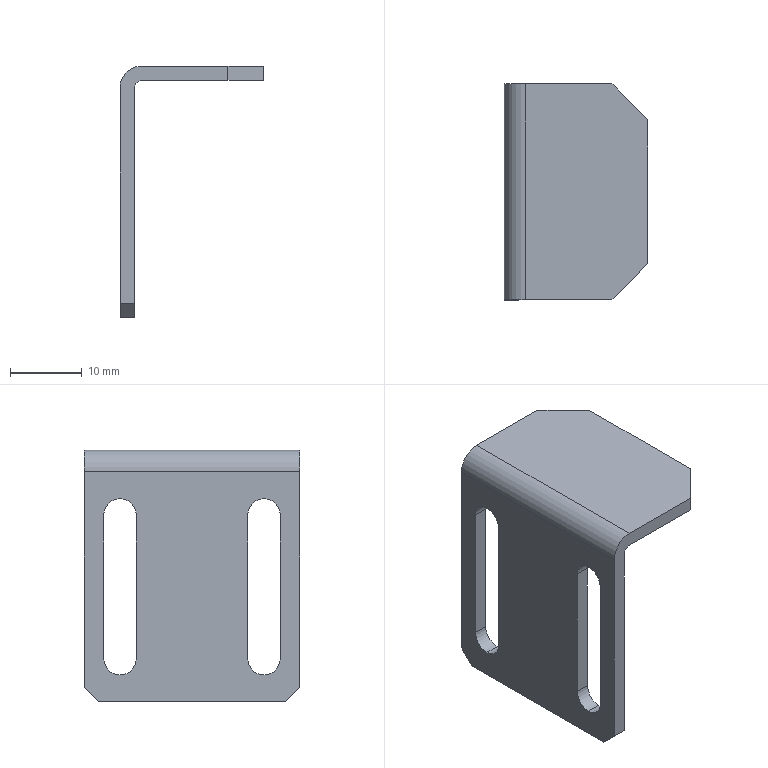Part | SolidWorks | features Chamfer 2, Fillet 2, ICE 2, Extrusion 1 | 1 solid | 24 faces | box 20 x 30 x 35 mm | volume 2647 mm3 | plane 16 | cylinder 8 | commonest cylinder face diameters 4.5 x6 2 x1 6 x1
STEP:
#1=CARTESIAN_POINT('',(0.,5.,-31.25));
#2=VERTEX_POINT('',#1);
#3=CARTESIAN_POINT('',(0.,7.25,-29.));
#4=VERTEX_POINT('',#3);
#5=CARTESIAN_POINT('',(0.,5.,-29.));
#6=DIRECTION('',(1.,0.,0.));
#7=DIRECTION('',(0.,0.,-1.));
#8=AXIS2_PLACEMENT_3D('',#5,#6,#7);
#9=CIRCLE('',#8,2.25);
#10=EDGE_CURVE('',#2,#4,#9,.T.);
#11=ORIENTED_EDGE('',*,*,#10,.F.);
#12=CARTESIAN_POINT('',(2.,5.,-31.25));
#13=VERTEX_POINT('',#12);
#14=CARTESIAN_POINT('',(-8.,5.,-31.25));
#15=DIRECTION('',(1.,0.,0.));
#16=VECTOR('',#15,1000.);
#17=LINE('',#14,#16);
#18=EDGE_CURVE('',#2,#13,#17,.T.);
#19=ORIENTED_EDGE('',*,*,#18,.T.);
#20=CARTESIAN_POINT('',(2.,7.25,-29.));
#21=VERTEX_POINT('',#20);
#22=CARTESIAN_POINT('',(2.,5.,-29.));
#23=DIRECTION('',(1.,0.,0.));
#24=DIRECTION('',(0.,0.,1.));
#25=AXIS2_PLACEMENT_3D('',#22,#23,#24);
#26=CIRCLE('',#25,2.25);
#27=EDGE_CURVE('',#13,#21,#26,.T.);
#28=ORIENTED_EDGE('',*,*,#27,.T.);
#29=CARTESIAN_POINT('',(-8.,7.25,-29.));
#30=DIRECTION('',(-1.,0.,0.));
#31=VECTOR('',#30,1000.);
#32=LINE('',#29,#31);
#33=EDGE_CURVE('',#21,#4,#32,.T.);
#34=ORIENTED_EDGE('',*,*,#33,.T.);
#35=EDGE_LOOP('',(#11,#19,#28,#34));
#36=FACE_OUTER_BOUND('',#35,.T.);
#37=CARTESIAN_POINT('',(-8.,5.,-29.));
#38=DIRECTION('',(1.,0.,0.));
#39=DIRECTION('',(0.,0.,-1.));
#40=AXIS2_PLACEMENT_3D('',#37,#38,#39);
#41=CYLINDRICAL_SURFACE('',#40,2.25);
#42=ADVANCED_FACE('',(#36),#41,.F.);
#43=CARTESIAN_POINT('',(0.,25.,-31.25));
#44=VERTEX_POINT('',#43);
#45=CARTESIAN_POINT('',(0.,27.25,-29.));
#46=VERTEX_POINT('',#45);
#47=CARTESIAN_POINT('',(0.,25.,-29.));
#48=DIRECTION('',(1.,0.,0.));
#49=DIRECTION('',(0.,0.,-1.));
#50=AXIS2_PLACEMENT_3D('',#47,#48,#49);
#51=CIRCLE('',#50,2.25);
#52=EDGE_CURVE('',#44,#46,#51,.T.);
#53=ORIENTED_EDGE('',*,*,#52,.F.);
#54=CARTESIAN_POINT('',(2.,25.,-31.25));
#55=VERTEX_POINT('',#54);
#56=CARTESIAN_POINT('',(-8.,25.,-31.25));
#57=DIRECTION('',(1.,0.,0.));
#58=VECTOR('',#57,1000.);
#59=LINE('',#56,#58);
#60=EDGE_CURVE('',#44,#55,#59,.T.);
#61=ORIENTED_EDGE('',*,*,#60,.T.);
#62=CARTESIAN_POINT('',(2.,27.25,-29.));
#63=VERTEX_POINT('',#62);
#64=CARTESIAN_POINT('',(2.,25.,-29.));
#65=DIRECTION('',(1.,0.,0.));
#66=DIRECTION('',(0.,0.,-1.));
#67=AXIS2_PLACEMENT_3D('',#64,#65,#66);
#68=CIRCLE('',#67,2.25);
#69=EDGE_CURVE('',#55,#63,#68,.T.);
#70=ORIENTED_EDGE('',*,*,#69,.T.);
#71=CARTESIAN_POINT('',(-8.,27.25,-29.));
#72=DIRECTION('',(-1.,0.,0.));
#73=VECTOR('',#72,1000.);
#74=LINE('',#71,#73);
#75=EDGE_CURVE('',#63,#46,#74,.T.);
#76=ORIENTED_EDGE('',*,*,#75,.T.);
#77=EDGE_LOOP('',(#53,#61,#70,#76));
#78=FACE_OUTER_BOUND('',#77,.T.);
#79=CARTESIAN_POINT('',(-8.,25.,-29.));
#80=DIRECTION('',(1.,0.,0.));
#81=DIRECTION('',(0.,0.,-1.));
#82=AXIS2_PLACEMENT_3D('',#79,#80,#81);
#83=CYLINDRICAL_SURFACE('',#82,2.25);
#84=ADVANCED_FACE('',(#78),#83,.F.);
#85=ORIENTED_EDGE('',*,*,#60,.F.);
#86=CARTESIAN_POINT('',(0.,22.75,-29.));
#87=VERTEX_POINT('',#86);
#88=CARTESIAN_POINT('',(0.,25.,-29.));
#89=DIRECTION('',(1.,0.,0.));
#90=DIRECTION('',(0.,0.,-1.));
#91=AXIS2_PLACEMENT_3D('',#88,#89,#90);
#92=CIRCLE('',#91,2.25);
#93=EDGE_CURVE('',#87,#44,#92,.T.);
#94=ORIENTED_EDGE('',*,*,#93,.F.);
#95=CARTESIAN_POINT('',(2.,22.75,-29.));
#96=VERTEX_POINT('',#95);
#97=CARTESIAN_POINT('',(-8.,22.75,-29.));
#98=DIRECTION('',(-1.,0.,0.));
#99=VECTOR('',#98,1000.);
#100=LINE('',#97,#99);
#101=EDGE_CURVE('',#96,#87,#100,.T.);
#102=ORIENTED_EDGE('',*,*,#101,.F.);
#103=CARTESIAN_POINT('',(2.,25.,-29.));
#104=DIRECTION('',(1.,0.,0.));
#105=DIRECTION('',(0.,0.,-1.));
#106=AXIS2_PLACEMENT_3D('',#103,#104,#105);
#107=CIRCLE('',#106,2.25);
#108=EDGE_CURVE('',#96,#55,#107,.T.);
#109=ORIENTED_EDGE('',*,*,#108,.T.);
#110=EDGE_LOOP('',(#85,#94,#102,#109));
#111=FACE_OUTER_BOUND('',#110,.T.);
#112=CARTESIAN_POINT('',(-8.,25.,-29.));
#113=DIRECTION('',(1.,0.,0.));
#114=DIRECTION('',(0.,0.,-1.));
#115=AXIS2_PLACEMENT_3D('',#112,#113,#114);
#116=CYLINDRICAL_SURFACE('',#115,2.25);
#117=ADVANCED_FACE('',(#111),#116,.F.);
#118=ORIENTED_EDGE('',*,*,#18,.F.);
#119=CARTESIAN_POINT('',(0.,2.75,-29.));
#120=VERTEX_POINT('',#119);
#121=CARTESIAN_POINT('',(0.,5.,-29.));
#122=DIRECTION('',(1.,0.,0.));
#123=DIRECTION('',(0.,0.,-1.));
#124=AXIS2_PLACEMENT_3D('',#121,#122,#123);
#125=CIRCLE('',#124,2.25);
#126=EDGE_CURVE('',#120,#2,#125,.T.);
#127=ORIENTED_EDGE('',*,*,#126,.F.);
#128=CARTESIAN_POINT('',(2.,2.75,-29.));
#129=VERTEX_POINT('',#128);
#130=CARTESIAN_POINT('',(-8.,2.75,-29.));
#131=DIRECTION('',(-1.,0.,0.));
#132=VECTOR('',#131,1000.);
#133=LINE('',#130,#132);
#134=EDGE_CURVE('',#129,#120,#133,.T.);
#135=ORIENTED_EDGE('',*,*,#134,.F.);
#136=CARTESIAN_POINT('',(2.,5.,-29.));
#137=DIRECTION('',(1.,0.,0.));
#138=DIRECTION('',(0.,0.,1.));
#139=AXIS2_PLACEMENT_3D('',#136,#137,#138);
#140=CIRCLE('',#139,2.25);
#141=EDGE_CURVE('',#129,#13,#140,.T.);
#142=ORIENTED_EDGE('',*,*,#141,.T.);
#143=EDGE_LOOP('',(#118,#127,#135,#142));
#144=FACE_OUTER_BOUND('',#143,.T.);
#145=CARTESIAN_POINT('',(-8.,5.,-29.));
#146=DIRECTION('',(1.,0.,0.));
#147=DIRECTION('',(0.,0.,-1.));
#148=AXIS2_PLACEMENT_3D('',#145,#146,#147);
#149=CYLINDRICAL_SURFACE('',#148,2.25);
#150=ADVANCED_FACE('',(#144),#149,.F.);
#151=CARTESIAN_POINT('',(0.,7.25,-9.));
#152=VERTEX_POINT('',#151);
#153=CARTESIAN_POINT('',(0.,2.75,-9.));
#154=VERTEX_POINT('',#153);
#155=CARTESIAN_POINT('',(0.,5.,-9.));
#156=DIRECTION('',(1.,0.,0.));
#157=DIRECTION('',(0.,0.,-1.));
#158=AXIS2_PLACEMENT_3D('',#155,#156,#157);
#159=CIRCLE('',#158,2.25);
#160=EDGE_CURVE('',#152,#154,#159,.T.);
#161=ORIENTED_EDGE('',*,*,#160,.T.);
#162=CARTESIAN_POINT('',(0.,2.75,0.));
#163=DIRECTION('',(0.,0.,-1.));
#164=VECTOR('',#163,1000.);
#165=LINE('',#162,#164);
#166=EDGE_CURVE('',#154,#120,#165,.T.);
#167=ORIENTED_EDGE('',*,*,#166,.T.);
#168=ORIENTED_EDGE('',*,*,#126,.T.);
#169=ORIENTED_EDGE('',*,*,#10,.T.);
#170=CARTESIAN_POINT('',(0.,7.25,0.));
#171=DIRECTION('',(0.,0.,1.));
#172=VECTOR('',#171,1000.);
#173=LINE('',#170,#172);
#174=EDGE_CURVE('',#4,#152,#173,.T.);
#175=ORIENTED_EDGE('',*,*,#174,.T.);
#176=EDGE_LOOP('',(#161,#167,#168,#169,#175));
#177=FACE_BOUND('',#176,.T.);
#178=CARTESIAN_POINT('',(0.,27.25,-9.));
#179=VERTEX_POINT('',#178);
#180=CARTESIAN_POINT('',(0.,22.75,-9.));
#181=VERTEX_POINT('',#180);
#182=CARTESIAN_POINT('',(0.,25.,-9.));
#183=DIRECTION('',(1.,0.,0.));
#184=DIRECTION('',(0.,0.,-1.));
#185=AXIS2_PLACEMENT_3D('',#182,#183,#184);
#186=CIRCLE('',#185,2.25);
#187=EDGE_CURVE('',#179,#181,#186,.T.);
#188=ORIENTED_EDGE('',*,*,#187,.T.);
#189=CARTESIAN_POINT('',(0.,22.75,0.));
#190=DIRECTION('',(0.,0.,-1.));
#191=VECTOR('',#190,1000.);
#192=LINE('',#189,#191);
#193=EDGE_CURVE('',#181,#87,#192,.T.);
#194=ORIENTED_EDGE('',*,*,#193,.T.);
#195=ORIENTED_EDGE('',*,*,#93,.T.);
#196=ORIENTED_EDGE('',*,*,#52,.T.);
#197=CARTESIAN_POINT('',(0.,27.25,0.));
#198=DIRECTION('',(0.,0.,1.));
#199=VECTOR('',#198,1000.);
#200=LINE('',#197,#199);
#201=EDGE_CURVE('',#46,#179,#200,.T.);
#202=ORIENTED_EDGE('',*,*,#201,.T.);
#203=EDGE_LOOP('',(#188,#194,#195,#196,#202));
#204=FACE_BOUND('',#203,.T.);
#205=CARTESIAN_POINT('',(0.,0.,-33.));
#206=VERTEX_POINT('',#205);
#207=CARTESIAN_POINT('',(0.,0.,-3.));
#208=VERTEX_POINT('',#207);
#209=CARTESIAN_POINT('',(0.,0.,0.));
#210=DIRECTION('',(0.,0.,1.));
#211=VECTOR('',#210,1000.);
#212=LINE('',#209,#211);
#213=EDGE_CURVE('',#206,#208,#212,.T.);
#214=ORIENTED_EDGE('',*,*,#213,.T.);
#215=CARTESIAN_POINT('',(0.,30.,-3.));
#216=VERTEX_POINT('',#215);
#217=CARTESIAN_POINT('',(0.,30.,-3.));
#218=DIRECTION('',(0.,1.,0.));
#219=VECTOR('',#218,1000.);
#220=LINE('',#217,#219);
#221=EDGE_CURVE('',#208,#216,#220,.T.);
#222=ORIENTED_EDGE('',*,*,#221,.T.);
#223=CARTESIAN_POINT('',(0.,30.,-33.));
#224=VERTEX_POINT('',#223);
#225=CARTESIAN_POINT('',(0.,30.,0.));
#226=DIRECTION('',(0.,0.,1.));
#227=VECTOR('',#226,1000.);
#228=LINE('',#225,#227);
#229=EDGE_CURVE('',#224,#216,#228,.T.);
#230=ORIENTED_EDGE('',*,*,#229,.F.);
#231=CARTESIAN_POINT('',(0.,28.,-35.));
#232=VERTEX_POINT('',#231);
#233=CARTESIAN_POINT('',(0.,30.,-33.));
#234=DIRECTION('',(0.,-0.7071,-0.7071));
#235=VECTOR('',#234,1000.);
#236=LINE('',#233,#235);
#237=EDGE_CURVE('',#224,#232,#236,.T.);
#238=ORIENTED_EDGE('',*,*,#237,.T.);
#239=CARTESIAN_POINT('',(0.,2.,-35.));
#240=VERTEX_POINT('',#239);
#241=CARTESIAN_POINT('',(0.,30.,-35.));
#242=DIRECTION('',(0.,-1.,0.));
#243=VECTOR('',#242,1000.);
#244=LINE('',#241,#243);
#245=EDGE_CURVE('',#232,#240,#244,.T.);
#246=ORIENTED_EDGE('',*,*,#245,.T.);
#247=CARTESIAN_POINT('',(0.,2.,-35.));
#248=DIRECTION('',(0.,-0.7071,0.7071));
#249=VECTOR('',#248,1000.);
#250=LINE('',#247,#249);
#251=EDGE_CURVE('',#240,#206,#250,.T.);
#252=ORIENTED_EDGE('',*,*,#251,.T.);
#253=EDGE_LOOP('',(#214,#222,#230,#238,#246,#252));
#254=FACE_OUTER_BOUND('',#253,.T.);
#255=CARTESIAN_POINT('',(0.,30.,0.));
#256=DIRECTION('',(1.,0.,0.));
#257=DIRECTION('',(0.,0.,-1.));
#258=AXIS2_PLACEMENT_3D('',#255,#256,#257);
#259=PLANE('',#258);
#260=ADVANCED_FACE('',(#177,#204,#254),#259,.F.);
#261=CARTESIAN_POINT('',(20.,25.,0.));
#262=VERTEX_POINT('',#261);
#263=CARTESIAN_POINT('',(20.,5.,0.));
#264=VERTEX_POINT('',#263);
#265=CARTESIAN_POINT('',(20.,30.,0.));
#266=DIRECTION('',(0.,-1.,0.));
#267=VECTOR('',#266,1000.);
#268=LINE('',#265,#267);
#269=EDGE_CURVE('',#262,#264,#268,.T.);
#270=ORIENTED_EDGE('',*,*,#269,.F.);
#271=CARTESIAN_POINT('',(15.,30.,0.));
#272=VERTEX_POINT('',#271);
#273=CARTESIAN_POINT('',(15.,30.,0.));
#274=DIRECTION('',(-0.7071,0.7071,0.));
#275=VECTOR('',#274,1000.);
#276=LINE('',#273,#275);
#277=EDGE_CURVE('',#262,#272,#276,.T.);
#278=ORIENTED_EDGE('',*,*,#277,.T.);
#279=CARTESIAN_POINT('',(3.,30.,0.));
#280=VERTEX_POINT('',#279);
#281=CARTESIAN_POINT('',(0.,30.,0.));
#282=DIRECTION('',(1.,0.,0.));
#283=VECTOR('',#282,1000.);
#284=LINE('',#281,#283);
#285=EDGE_CURVE('',#280,#272,#284,.T.);
#286=ORIENTED_EDGE('',*,*,#285,.F.);
#287=CARTESIAN_POINT('',(3.,0.,0.));
#288=VERTEX_POINT('',#287);
#289=CARTESIAN_POINT('',(3.,30.,0.));
#290=DIRECTION('',(0.,-1.,0.));
#291=VECTOR('',#290,1000.);
#292=LINE('',#289,#291);
#293=EDGE_CURVE('',#280,#288,#292,.T.);
#294=ORIENTED_EDGE('',*,*,#293,.T.);
#295=CARTESIAN_POINT('',(15.,0.,0.));
#296=VERTEX_POINT('',#295);
#297=CARTESIAN_POINT('',(0.,0.,0.));
#298=DIRECTION('',(1.,0.,0.));
#299=VECTOR('',#298,1000.);
#300=LINE('',#297,#299);
#301=EDGE_CURVE('',#288,#296,#300,.T.);
#302=ORIENTED_EDGE('',*,*,#301,.T.);
#303=CARTESIAN_POINT('',(20.,5.,0.));
#304=DIRECTION('',(0.7071,0.7071,0.));
#305=VECTOR('',#304,1000.);
#306=LINE('',#303,#305);
#307=EDGE_CURVE('',#296,#264,#306,.T.);
#308=ORIENTED_EDGE('',*,*,#307,.T.);
#309=EDGE_LOOP('',(#270,#278,#286,#294,#302,#308));
#310=FACE_OUTER_BOUND('',#309,.T.);
#311=CARTESIAN_POINT('',(0.,30.,0.));
#312=DIRECTION('',(0.,0.,-1.));
#313=DIRECTION('',(-1.,0.,0.));
#314=AXIS2_PLACEMENT_3D('',#311,#312,#313);
#315=PLANE('',#314);
#316=ADVANCED_FACE('',(#310),#315,.F.);
#317=CARTESIAN_POINT('',(20.,25.,-2.));
#318=VERTEX_POINT('',#317);
#319=CARTESIAN_POINT('',(20.,5.,-2.));
#320=VERTEX_POINT('',#319);
#321=CARTESIAN_POINT('',(20.,30.,-2.));
#322=DIRECTION('',(0.,-1.,0.));
#323=VECTOR('',#322,1000.);
#324=LINE('',#321,#323);
#325=EDGE_CURVE('',#318,#320,#324,.T.);
#326=ORIENTED_EDGE('',*,*,#325,.F.);
#327=CARTESIAN_POINT('',(20.,25.,0.));
#328=DIRECTION('',(0.,0.,1.));
#329=VECTOR('',#328,1000.);
#330=LINE('',#327,#329);
#331=EDGE_CURVE('',#318,#262,#330,.T.);
#332=ORIENTED_EDGE('',*,*,#331,.T.);
#333=ORIENTED_EDGE('',*,*,#269,.T.);
#334=CARTESIAN_POINT('',(20.,5.,-2.));
#335=DIRECTION('',(0.,0.,-1.));
#336=VECTOR('',#335,1000.);
#337=LINE('',#334,#336);
#338=EDGE_CURVE('',#264,#320,#337,.T.);
#339=ORIENTED_EDGE('',*,*,#338,.T.);
#340=EDGE_LOOP('',(#326,#332,#333,#339));
#341=FACE_OUTER_BOUND('',#340,.T.);
#342=CARTESIAN_POINT('',(20.,30.,0.));
#343=DIRECTION('',(-1.,0.,0.));
#344=DIRECTION('',(0.,0.,1.));
#345=AXIS2_PLACEMENT_3D('',#342,#343,#344);
#346=PLANE('',#345);
#347=ADVANCED_FACE('',(#341),#346,.F.);
#348=CARTESIAN_POINT('',(15.,30.,-2.));
#349=VERTEX_POINT('',#348);
#350=CARTESIAN_POINT('',(3.,30.,-2.));
#351=VERTEX_POINT('',#350);
#352=CARTESIAN_POINT('',(20.,30.,-2.));
#353=DIRECTION('',(-1.,0.,0.));
#354=VECTOR('',#353,1000.);
#355=LINE('',#352,#354);
#356=EDGE_CURVE('',#349,#351,#355,.T.);
#357=ORIENTED_EDGE('',*,*,#356,.F.);
#358=CARTESIAN_POINT('',(15.,30.,-2.));
#359=DIRECTION('',(0.7071,-0.7071,0.));
#360=VECTOR('',#359,1000.);
#361=LINE('',#358,#360);
#362=EDGE_CURVE('',#349,#318,#361,.T.);
#363=ORIENTED_EDGE('',*,*,#362,.T.);
#364=ORIENTED_EDGE('',*,*,#325,.T.);
#365=CARTESIAN_POINT('',(15.,0.,-2.));
#366=VERTEX_POINT('',#365);
#367=CARTESIAN_POINT('',(20.,5.,-2.));
#368=DIRECTION('',(-0.7071,-0.7071,0.));
#369=VECTOR('',#368,1000.);
#370=LINE('',#367,#369);
#371=EDGE_CURVE('',#320,#366,#370,.T.);
#372=ORIENTED_EDGE('',*,*,#371,.T.);
#373=CARTESIAN_POINT('',(3.,0.,-2.));
#374=VERTEX_POINT('',#373);
#375=CARTESIAN_POINT('',(20.,0.,-2.));
#376=DIRECTION('',(-1.,0.,0.));
#377=VECTOR('',#376,1000.);
#378=LINE('',#375,#377);
#379=EDGE_CURVE('',#366,#374,#378,.T.);
#380=ORIENTED_EDGE('',*,*,#379,.T.);
#381=CARTESIAN_POINT('',(3.,30.,-2.));
#382=DIRECTION('',(0.,1.,0.));
#383=VECTOR('',#382,1000.);
#384=LINE('',#381,#383);
#385=EDGE_CURVE('',#374,#351,#384,.T.);
#386=ORIENTED_EDGE('',*,*,#385,.T.);
#387=EDGE_LOOP('',(#357,#363,#364,#372,#380,#386));
#388=FACE_OUTER_BOUND('',#387,.T.);
#389=CARTESIAN_POINT('',(20.,30.,-2.));
#390=DIRECTION('',(0.,0.,1.));
#391=DIRECTION('',(1.,0.,0.));
#392=AXIS2_PLACEMENT_3D('',#389,#390,#391);
#393=PLANE('',#392);
#394=ADVANCED_FACE('',(#388),#393,.F.);
#395=ORIENTED_EDGE('',*,*,#141,.F.);
#396=CARTESIAN_POINT('',(2.,2.75,-9.));
#397=VERTEX_POINT('',#396);
#398=CARTESIAN_POINT('',(2.,2.75,-29.));
#399=DIRECTION('',(0.,0.,-1.));
#400=VECTOR('',#399,1000.);
#401=LINE('',#398,#400);
#402=EDGE_CURVE('',#397,#129,#401,.T.);
#403=ORIENTED_EDGE('',*,*,#402,.F.);
#404=CARTESIAN_POINT('',(2.,7.25,-9.));
#405=VERTEX_POINT('',#404);
#406=CARTESIAN_POINT('',(2.,5.,-9.));
#407=DIRECTION('',(1.,0.,0.));
#408=DIRECTION('',(0.,0.,-1.));
#409=AXIS2_PLACEMENT_3D('',#406,#407,#408);
#410=CIRCLE('',#409,2.25);
#411=EDGE_CURVE('',#405,#397,#410,.T.);
#412=ORIENTED_EDGE('',*,*,#411,.F.);
#413=CARTESIAN_POINT('',(2.,7.25,-29.));
#414=DIRECTION('',(0.,0.,1.));
#415=VECTOR('',#414,1000.);
#416=LINE('',#413,#415);
#417=EDGE_CURVE('',#21,#405,#416,.T.);
#418=ORIENTED_EDGE('',*,*,#417,.F.);
#419=ORIENTED_EDGE('',*,*,#27,.F.);
#420=EDGE_LOOP('',(#395,#403,#412,#418,#419));
#421=FACE_BOUND('',#420,.T.);
#422=ORIENTED_EDGE('',*,*,#108,.F.);
#423=CARTESIAN_POINT('',(2.,22.75,-9.));
#424=VERTEX_POINT('',#423);
#425=CARTESIAN_POINT('',(2.,22.75,-29.));
#426=DIRECTION('',(0.,0.,-1.));
#427=VECTOR('',#426,1000.);
#428=LINE('',#425,#427);
#429=EDGE_CURVE('',#424,#96,#428,.T.);
#430=ORIENTED_EDGE('',*,*,#429,.F.);
#431=CARTESIAN_POINT('',(2.,27.25,-9.));
#432=VERTEX_POINT('',#431);
#433=CARTESIAN_POINT('',(2.,25.,-9.));
#434=DIRECTION('',(1.,0.,0.));
#435=DIRECTION('',(0.,0.,1.));
#436=AXIS2_PLACEMENT_3D('',#433,#434,#435);
#437=CIRCLE('',#436,2.25);
#438=EDGE_CURVE('',#432,#424,#437,.T.);
#439=ORIENTED_EDGE('',*,*,#438,.F.);
#440=CARTESIAN_POINT('',(2.,27.25,-29.));
#441=DIRECTION('',(0.,0.,1.));
#442=VECTOR('',#441,1000.);
#443=LINE('',#440,#442);
#444=EDGE_CURVE('',#63,#432,#443,.T.);
#445=ORIENTED_EDGE('',*,*,#444,.F.);
#446=ORIENTED_EDGE('',*,*,#69,.F.);
#447=EDGE_LOOP('',(#422,#430,#439,#445,#446));
#448=FACE_BOUND('',#447,.T.);
#449=CARTESIAN_POINT('',(2.,30.,-3.));
#450=VERTEX_POINT('',#449);
#451=CARTESIAN_POINT('',(2.,30.,-33.));
#452=VERTEX_POINT('',#451);
#453=CARTESIAN_POINT('',(2.,30.,-35.));
#454=DIRECTION('',(0.,0.,-1.));
#455=VECTOR('',#454,1000.);
#456=LINE('',#453,#455);
#457=EDGE_CURVE('',#450,#452,#456,.T.);
#458=ORIENTED_EDGE('',*,*,#457,.F.);
#459=CARTESIAN_POINT('',(2.,0.,-3.));
#460=VERTEX_POINT('',#459);
#461=CARTESIAN_POINT('',(2.,0.,-3.));
#462=DIRECTION('',(0.,-1.,0.));
#463=VECTOR('',#462,1000.);
#464=LINE('',#461,#463);
#465=EDGE_CURVE('',#450,#460,#464,.T.);
#466=ORIENTED_EDGE('',*,*,#465,.T.);
#467=CARTESIAN_POINT('',(2.,0.,-33.));
#468=VERTEX_POINT('',#467);
#469=CARTESIAN_POINT('',(2.,0.,-35.));
#470=DIRECTION('',(0.,0.,-1.));
#471=VECTOR('',#470,1000.);
#472=LINE('',#469,#471);
#473=EDGE_CURVE('',#460,#468,#472,.T.);
#474=ORIENTED_EDGE('',*,*,#473,.T.);
#475=CARTESIAN_POINT('',(2.,2.,-35.));
#476=VERTEX_POINT('',#475);
#477=CARTESIAN_POINT('',(2.,2.,-35.));
#478=DIRECTION('',(0.,0.7071,-0.7071));
#479=VECTOR('',#478,1000.);
#480=LINE('',#477,#479);
#481=EDGE_CURVE('',#468,#476,#480,.T.);
#482=ORIENTED_EDGE('',*,*,#481,.T.);
#483=CARTESIAN_POINT('',(2.,28.,-35.));
#484=VERTEX_POINT('',#483);
#485=CARTESIAN_POINT('',(2.,30.,-35.));
#486=DIRECTION('',(0.,-1.,0.));
#487=VECTOR('',#486,1000.);
#488=LINE('',#485,#487);
#489=EDGE_CURVE('',#484,#476,#488,.T.);
#490=ORIENTED_EDGE('',*,*,#489,.F.);
#491=CARTESIAN_POINT('',(2.,30.,-33.));
#492=DIRECTION('',(0.,0.7071,0.7071));
#493=VECTOR('',#492,1000.);
#494=LINE('',#491,#493);
#495=EDGE_CURVE('',#484,#452,#494,.T.);
#496=ORIENTED_EDGE('',*,*,#495,.T.);
#497=EDGE_LOOP('',(#458,#466,#474,#482,#490,#496));
#498=FACE_OUTER_BOUND('',#497,.T.);
#499=CARTESIAN_POINT('',(2.,30.,-35.));
#500=DIRECTION('',(-1.,0.,0.));
#501=DIRECTION('',(0.,0.,1.));
#502=AXIS2_PLACEMENT_3D('',#499,#500,#501);
#503=PLANE('',#502);
#504=ADVANCED_FACE('',(#421,#448,#498),#503,.F.);
#505=ORIENTED_EDGE('',*,*,#245,.F.);
#506=CARTESIAN_POINT('',(0.,28.,-35.));
#507=DIRECTION('',(1.,0.,0.));
#508=VECTOR('',#507,1000.);
#509=LINE('',#506,#508);
#510=EDGE_CURVE('',#232,#484,#509,.T.);
#511=ORIENTED_EDGE('',*,*,#510,.T.);
#512=ORIENTED_EDGE('',*,*,#489,.T.);
#513=CARTESIAN_POINT('',(0.,2.,-35.));
#514=DIRECTION('',(-1.,0.,0.));
#515=VECTOR('',#514,1000.);
#516=LINE('',#513,#515);
#517=EDGE_CURVE('',#476,#240,#516,.T.);
#518=ORIENTED_EDGE('',*,*,#517,.T.);
#519=EDGE_LOOP('',(#505,#511,#512,#518));
#520=FACE_OUTER_BOUND('',#519,.T.);
#521=CARTESIAN_POINT('',(0.,30.,-35.));
#522=DIRECTION('',(0.,0.,1.));
#523=DIRECTION('',(1.,0.,0.));
#524=AXIS2_PLACEMENT_3D('',#521,#522,#523);
#525=PLANE('',#524);
#526=ADVANCED_FACE('',(#520),#525,.F.);
#527=ORIENTED_EDGE('',*,*,#285,.T.);
#528=CARTESIAN_POINT('',(15.,30.,0.));
#529=DIRECTION('',(0.,0.,-1.));
#530=VECTOR('',#529,1000.);
#531=LINE('',#528,#530);
#532=EDGE_CURVE('',#272,#349,#531,.T.);
#533=ORIENTED_EDGE('',*,*,#532,.T.);
#534=ORIENTED_EDGE('',*,*,#356,.T.);
#535=CARTESIAN_POINT('',(3.,30.,-3.));
#536=DIRECTION('',(0.,-1.,0.));
#537=DIRECTION('',(0.,0.,-1.));
#538=AXIS2_PLACEMENT_3D('',#535,#536,#537);
#539=CIRCLE('',#538,1.);
#540=EDGE_CURVE('',#351,#450,#539,.T.);
#541=ORIENTED_EDGE('',*,*,#540,.T.);
#542=ORIENTED_EDGE('',*,*,#457,.T.);
#543=CARTESIAN_POINT('',(0.,30.,-33.));
#544=DIRECTION('',(-1.,0.,0.));
#545=VECTOR('',#544,1000.);
#546=LINE('',#543,#545);
#547=EDGE_CURVE('',#452,#224,#546,.T.);
#548=ORIENTED_EDGE('',*,*,#547,.T.);
#549=ORIENTED_EDGE('',*,*,#229,.T.);
#550=CARTESIAN_POINT('',(3.,30.,-3.));
#551=DIRECTION('',(0.,1.,0.));
#552=DIRECTION('',(0.,0.,-1.));
#553=AXIS2_PLACEMENT_3D('',#550,#551,#552);
#554=CIRCLE('',#553,3.);
#555=EDGE_CURVE('',#216,#280,#554,.T.);
#556=ORIENTED_EDGE('',*,*,#555,.T.);
#557=EDGE_LOOP('',(#527,#533,#534,#541,#542,#548,#549,#556));
#558=FACE_OUTER_BOUND('',#557,.T.);
#559=CARTESIAN_POINT('',(0.,30.,0.));
#560=DIRECTION('',(0.,-1.,0.));
#561=DIRECTION('',(0.,0.,-1.));
#562=AXIS2_PLACEMENT_3D('',#559,#560,#561);
#563=PLANE('',#562);
#564=ADVANCED_FACE('',(#558),#563,.F.);
#565=ORIENTED_EDGE('',*,*,#379,.F.);
#566=CARTESIAN_POINT('',(15.,0.,0.));
#567=DIRECTION('',(0.,0.,1.));
#568=VECTOR('',#567,1000.);
#569=LINE('',#566,#568);
#570=EDGE_CURVE('',#366,#296,#569,.T.);
#571=ORIENTED_EDGE('',*,*,#570,.T.);
#572=ORIENTED_EDGE('',*,*,#301,.F.);
#573=CARTESIAN_POINT('',(3.,0.,-3.));
#574=DIRECTION('',(0.,-1.,0.));
#575=DIRECTION('',(0.,0.,-1.));
#576=AXIS2_PLACEMENT_3D('',#573,#574,#575);
#577=CIRCLE('',#576,3.);
#578=EDGE_CURVE('',#288,#208,#577,.T.);
#579=ORIENTED_EDGE('',*,*,#578,.T.);
#580=ORIENTED_EDGE('',*,*,#213,.F.);
#581=CARTESIAN_POINT('',(2.,0.,-33.));
#582=DIRECTION('',(1.,0.,0.));
#583=VECTOR('',#582,1000.);
#584=LINE('',#581,#583);
#585=EDGE_CURVE('',#206,#468,#584,.T.);
#586=ORIENTED_EDGE('',*,*,#585,.T.);
#587=ORIENTED_EDGE('',*,*,#473,.F.);
#588=CARTESIAN_POINT('',(3.,0.,-3.));
#589=DIRECTION('',(0.,1.,0.));
#590=DIRECTION('',(0.,0.,-1.));
#591=AXIS2_PLACEMENT_3D('',#588,#589,#590);
#592=CIRCLE('',#591,1.);
#593=EDGE_CURVE('',#460,#374,#592,.T.);
#594=ORIENTED_EDGE('',*,*,#593,.T.);
#595=EDGE_LOOP('',(#565,#571,#572,#579,#580,#586,#587,#594));
#596=FACE_OUTER_BOUND('',#595,.T.);
#597=CARTESIAN_POINT('',(0.,0.,0.));
#598=DIRECTION('',(0.,-1.,0.));
#599=DIRECTION('',(0.,0.,-1.));
#600=AXIS2_PLACEMENT_3D('',#597,#598,#599);
#601=PLANE('',#600);
#602=ADVANCED_FACE('',(#596),#601,.T.);
#603=ORIENTED_EDGE('',*,*,#495,.F.);
#604=ORIENTED_EDGE('',*,*,#510,.F.);
#605=ORIENTED_EDGE('',*,*,#237,.F.);
#606=ORIENTED_EDGE('',*,*,#547,.F.);
#607=EDGE_LOOP('',(#603,#604,#605,#606));
#608=FACE_OUTER_BOUND('',#607,.T.);
#609=CARTESIAN_POINT('',(0.,30.,-33.));
#610=DIRECTION('',(0.,-0.7071,0.7071));
#611=DIRECTION('',(-1.,0.,0.));
#612=AXIS2_PLACEMENT_3D('',#609,#610,#611);
#613=PLANE('',#612);
#614=ADVANCED_FACE('',(#608),#613,.F.);
#615=ORIENTED_EDGE('',*,*,#481,.F.);
#616=ORIENTED_EDGE('',*,*,#585,.F.);
#617=ORIENTED_EDGE('',*,*,#251,.F.);
#618=ORIENTED_EDGE('',*,*,#517,.F.);
#619=EDGE_LOOP('',(#615,#616,#617,#618));
#620=FACE_OUTER_BOUND('',#619,.T.);
#621=CARTESIAN_POINT('',(0.,2.,-35.));
#622=DIRECTION('',(0.,-0.7071,-0.7071));
#623=DIRECTION('',(1.,0.,0.));
#624=AXIS2_PLACEMENT_3D('',#621,#622,#623);
#625=PLANE('',#624);
#626=ADVANCED_FACE('',(#620),#625,.T.);
#627=ORIENTED_EDGE('',*,*,#540,.F.);
#628=ORIENTED_EDGE('',*,*,#385,.F.);
#629=ORIENTED_EDGE('',*,*,#593,.F.);
#630=ORIENTED_EDGE('',*,*,#465,.F.);
#631=EDGE_LOOP('',(#627,#628,#629,#630));
#632=FACE_OUTER_BOUND('',#631,.T.);
#633=CARTESIAN_POINT('',(3.,30.,-3.));
#634=DIRECTION('',(0.,1.,0.));
#635=DIRECTION('',(0.,0.,1.));
#636=AXIS2_PLACEMENT_3D('',#633,#634,#635);
#637=CYLINDRICAL_SURFACE('',#636,1.);
#638=ADVANCED_FACE('',(#632),#637,.F.);
#639=ORIENTED_EDGE('',*,*,#555,.F.);
#640=ORIENTED_EDGE('',*,*,#221,.F.);
#641=ORIENTED_EDGE('',*,*,#578,.F.);
#642=ORIENTED_EDGE('',*,*,#293,.F.);
#643=EDGE_LOOP('',(#639,#640,#641,#642));
#644=FACE_OUTER_BOUND('',#643,.T.);
#645=CARTESIAN_POINT('',(3.,30.,-3.));
#646=DIRECTION('',(0.,-1.,0.));
#647=DIRECTION('',(0.,0.,-1.));
#648=AXIS2_PLACEMENT_3D('',#645,#646,#647);
#649=CYLINDRICAL_SURFACE('',#648,3.);
#650=ADVANCED_FACE('',(#644),#649,.T.);
#651=ORIENTED_EDGE('',*,*,#277,.F.);
#652=ORIENTED_EDGE('',*,*,#331,.F.);
#653=ORIENTED_EDGE('',*,*,#362,.F.);
#654=ORIENTED_EDGE('',*,*,#532,.F.);
#655=EDGE_LOOP('',(#651,#652,#653,#654));
#656=FACE_OUTER_BOUND('',#655,.T.);
#657=CARTESIAN_POINT('',(15.,30.,0.));
#658=DIRECTION('',(-0.7071,-0.7071,0.));
#659=DIRECTION('',(0.,0.,-1.));
#660=AXIS2_PLACEMENT_3D('',#657,#658,#659);
#661=PLANE('',#660);
#662=ADVANCED_FACE('',(#656),#661,.F.);
#663=ORIENTED_EDGE('',*,*,#307,.F.);
#664=ORIENTED_EDGE('',*,*,#570,.F.);
#665=ORIENTED_EDGE('',*,*,#371,.F.);
#666=ORIENTED_EDGE('',*,*,#338,.F.);
#667=EDGE_LOOP('',(#663,#664,#665,#666));
#668=FACE_OUTER_BOUND('',#667,.T.);
#669=CARTESIAN_POINT('',(20.,5.,0.));
#670=DIRECTION('',(0.7071,-0.7071,0.));
#671=DIRECTION('',(0.,0.,1.));
#672=AXIS2_PLACEMENT_3D('',#669,#670,#671);
#673=PLANE('',#672);
#674=ADVANCED_FACE('',(#668),#673,.T.);
#675=CARTESIAN_POINT('',(-8.,7.25,-9.));
#676=DIRECTION('',(1.,0.,0.));
#677=VECTOR('',#676,1000.);
#678=LINE('',#675,#677);
#679=EDGE_CURVE('',#152,#405,#678,.T.);
#680=ORIENTED_EDGE('',*,*,#679,.T.);
#681=ORIENTED_EDGE('',*,*,#411,.T.);
#682=CARTESIAN_POINT('',(-8.,2.75,-9.));
#683=DIRECTION('',(1.,0.,0.));
#684=VECTOR('',#683,1000.);
#685=LINE('',#682,#684);
#686=EDGE_CURVE('',#154,#397,#685,.T.);
#687=ORIENTED_EDGE('',*,*,#686,.F.);
#688=ORIENTED_EDGE('',*,*,#160,.F.);
#689=EDGE_LOOP('',(#680,#681,#687,#688));
#690=FACE_OUTER_BOUND('',#689,.T.);
#691=CARTESIAN_POINT('',(-8.,5.,-9.));
#692=DIRECTION('',(1.,0.,0.));
#693=DIRECTION('',(0.,0.,-1.));
#694=AXIS2_PLACEMENT_3D('',#691,#692,#693);
#695=CYLINDRICAL_SURFACE('',#694,2.25);
#696=ADVANCED_FACE('',(#690),#695,.F.);
#697=ORIENTED_EDGE('',*,*,#686,.T.);
#698=ORIENTED_EDGE('',*,*,#402,.T.);
#699=ORIENTED_EDGE('',*,*,#134,.T.);
#700=ORIENTED_EDGE('',*,*,#166,.F.);
#701=EDGE_LOOP('',(#697,#698,#699,#700));
#702=FACE_OUTER_BOUND('',#701,.T.);
#703=CARTESIAN_POINT('',(-8.,2.75,-29.));
#704=DIRECTION('',(0.,-1.,0.));
#705=DIRECTION('',(0.,0.,-1.));
#706=AXIS2_PLACEMENT_3D('',#703,#704,#705);
#707=PLANE('',#706);
#708=ADVANCED_FACE('',(#702),#707,.F.);
#709=ORIENTED_EDGE('',*,*,#33,.F.);
#710=ORIENTED_EDGE('',*,*,#417,.T.);
#711=ORIENTED_EDGE('',*,*,#679,.F.);
#712=ORIENTED_EDGE('',*,*,#174,.F.);
#713=EDGE_LOOP('',(#709,#710,#711,#712));
#714=FACE_OUTER_BOUND('',#713,.T.);
#715=CARTESIAN_POINT('',(-8.,7.25,-29.));
#716=DIRECTION('',(0.,1.,0.));
#717=DIRECTION('',(0.,0.,1.));
#718=AXIS2_PLACEMENT_3D('',#715,#716,#717);
#719=PLANE('',#718);
#720=ADVANCED_FACE('',(#714),#719,.F.);
#721=CARTESIAN_POINT('',(-8.,27.25,-9.));
#722=DIRECTION('',(1.,0.,0.));
#723=VECTOR('',#722,1000.);
#724=LINE('',#721,#723);
#725=EDGE_CURVE('',#179,#432,#724,.T.);
#726=ORIENTED_EDGE('',*,*,#725,.T.);
#727=ORIENTED_EDGE('',*,*,#438,.T.);
#728=CARTESIAN_POINT('',(-8.,22.75,-9.));
#729=DIRECTION('',(1.,0.,0.));
#730=VECTOR('',#729,1000.);
#731=LINE('',#728,#730);
#732=EDGE_CURVE('',#181,#424,#731,.T.);
#733=ORIENTED_EDGE('',*,*,#732,.F.);
#734=ORIENTED_EDGE('',*,*,#187,.F.);
#735=EDGE_LOOP('',(#726,#727,#733,#734));
#736=FACE_OUTER_BOUND('',#735,.T.);
#737=CARTESIAN_POINT('',(-8.,25.,-9.));
#738=DIRECTION('',(1.,0.,0.));
#739=DIRECTION('',(0.,0.,-1.));
#740=AXIS2_PLACEMENT_3D('',#737,#738,#739);
#741=CYLINDRICAL_SURFACE('',#740,2.25);
#742=ADVANCED_FACE('',(#736),#741,.F.);
#743=ORIENTED_EDGE('',*,*,#732,.T.);
#744=ORIENTED_EDGE('',*,*,#429,.T.);
#745=ORIENTED_EDGE('',*,*,#101,.T.);
#746=ORIENTED_EDGE('',*,*,#193,.F.);
#747=EDGE_LOOP('',(#743,#744,#745,#746));
#748=FACE_OUTER_BOUND('',#747,.T.);
#749=CARTESIAN_POINT('',(-8.,22.75,-29.));
#750=DIRECTION('',(0.,-1.,0.));
#751=DIRECTION('',(0.,0.,-1.));
#752=AXIS2_PLACEMENT_3D('',#749,#750,#751);
#753=PLANE('',#752);
#754=ADVANCED_FACE('',(#748),#753,.F.);
#755=ORIENTED_EDGE('',*,*,#75,.F.);
#756=ORIENTED_EDGE('',*,*,#444,.T.);
#757=ORIENTED_EDGE('',*,*,#725,.F.);
#758=ORIENTED_EDGE('',*,*,#201,.F.);
#759=EDGE_LOOP('',(#755,#756,#757,#758));
#760=FACE_OUTER_BOUND('',#759,.T.);
#761=CARTESIAN_POINT('',(-8.,27.25,-29.));
#762=DIRECTION('',(0.,1.,0.));
#763=DIRECTION('',(0.,0.,1.));
#764=AXIS2_PLACEMENT_3D('',#761,#762,#763);
#765=PLANE('',#764);
#766=ADVANCED_FACE('',(#760),#765,.F.);
#767=CLOSED_SHELL('',(#42,#84,#117,#150,#260,#316,#347,#394,#504,#526,#564,#602,#614,#626,#638,#650,#662,#674,#696,#708,#720,#742,#754,#766));
#768=MANIFOLD_SOLID_BREP('',#767);
#769=CARTESIAN_POINT('',(0.,0.,0.));
#770=DIRECTION('',(0.,0.,1.));
#771=DIRECTION('',(1.,0.,0.));
#772=AXIS2_PLACEMENT_3D('',#769,#770,#771);
#773=(LENGTH_UNIT()NAMED_UNIT(*)SI_UNIT(.MILLI.,.METRE.));
#774=UNCERTAINTY_MEASURE_WITH_UNIT(LENGTH_MEASURE(0.00001),#773,'','');
#775=(NAMED_UNIT(*)PLANE_ANGLE_UNIT()SI_UNIT($,.RADIAN.));
#776=(NAMED_UNIT(*)SI_UNIT($,.STERADIAN.)SOLID_ANGLE_UNIT());
#777=(GEOMETRIC_REPRESENTATION_CONTEXT(3)GLOBAL_UNCERTAINTY_ASSIGNED_CONTEXT((#774))GLOBAL_UNIT_ASSIGNED_CONTEXT((#773,#775,#776))REPRESENTATION_CONTEXT('',''));
#778=ADVANCED_BREP_SHAPE_REPRESENTATION('',(#768,#772),#777);